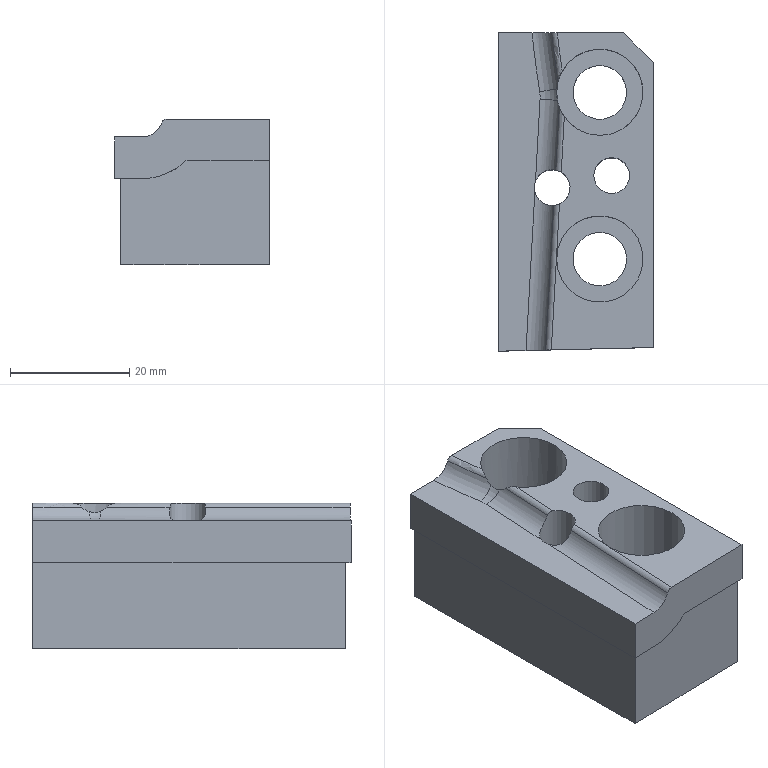Part | NX | features solid 2 | 1 solid | 27 faces | box 26 x 53.487 x 24.5 mm | volume 23516 mm3 | plane 12 | cylinder 10 | torus 3 | spline 2 | commonest cylinder face diameters 2 x2 6.001 x2 7 x2 9 x2 14.5 x2
STEP:
#1=CARTESIAN_POINT('',(636.878,-88.728,-8.5));
#2=VERTEX_POINT('',#1);
#3=CARTESIAN_POINT('',(636.878,-88.728,-23.));
#4=VERTEX_POINT('',#3);
#5=CARTESIAN_POINT('',(636.878,-88.728,-58.5));
#6=DIRECTION('',(0.,0.,1.));
#7=VECTOR('',#6,1000.);
#8=LINE('',#5,#7);
#9=EDGE_CURVE('',#2,#4,#8,.F.);
#10=ORIENTED_EDGE('',*,*,#9,.F.);
#11=CARTESIAN_POINT('',(636.878,-36.265,-8.5));
#12=VERTEX_POINT('',#11);
#13=CARTESIAN_POINT('',(636.878,-73.265,-8.5));
#14=DIRECTION('',(0.,-1.,0.));
#15=VECTOR('',#14,1000.);
#16=LINE('',#13,#15);
#17=EDGE_CURVE('',#12,#2,#16,.T.);
#18=ORIENTED_EDGE('',*,*,#17,.F.);
#19=CARTESIAN_POINT('',(636.878,-36.265,-23.));
#20=VERTEX_POINT('',#19);
#21=CARTESIAN_POINT('',(636.878,-36.265,-5.));
#22=DIRECTION('',(0.,0.,1.));
#23=VECTOR('',#22,1000.);
#24=LINE('',#21,#23);
#25=EDGE_CURVE('',#20,#12,#24,.T.);
#26=ORIENTED_EDGE('',*,*,#25,.F.);
#27=CARTESIAN_POINT('',(636.878,-73.265,-23.));
#28=DIRECTION('',(0.,1.,0.));
#29=VECTOR('',#28,1000.);
#30=LINE('',#27,#29);
#31=EDGE_CURVE('',#20,#4,#30,.F.);
#32=ORIENTED_EDGE('',*,*,#31,.T.);
#33=EDGE_LOOP('',(#10,#18,#26,#32));
#34=FACE_BOUND('',#33,.T.);
#35=CARTESIAN_POINT('',(636.878,-73.265,-5.));
#36=DIRECTION('',(1.,0.,0.));
#37=DIRECTION('',(0.,0.,-1.));
#38=AXIS2_PLACEMENT_3D('',#35,#36,#37);
#39=PLANE('',#38);
#40=ADVANCED_FACE('',(#34),#39,.F.);
#41=CARTESIAN_POINT('',(635.878,-89.752,-8.5));
#42=VERTEX_POINT('',#41);
#43=CARTESIAN_POINT('',(635.878,-89.752,-1.5));
#44=VERTEX_POINT('',#43);
#45=CARTESIAN_POINT('',(635.878,-89.752,22.));
#46=DIRECTION('',(0.,0.,1.));
#47=VECTOR('',#46,1000.);
#48=LINE('',#45,#47);
#49=EDGE_CURVE('',#42,#44,#48,.T.);
#50=ORIENTED_EDGE('',*,*,#49,.F.);
#51=CARTESIAN_POINT('',(661.878,-89.14,-5.5));
#52=VERTEX_POINT('',#51);
#53=CARTESIAN_POINT('',(635.878,-89.752,-8.5));
#54=CARTESIAN_POINT('',(636.986,-89.726,-8.499));
#55=CARTESIAN_POINT('',(639.207,-89.674,-8.501));
#56=CARTESIAN_POINT('',(641.968,-89.609,-8.497));
#57=CARTESIAN_POINT('',(643.879,-89.564,-7.982));
#58=CARTESIAN_POINT('',(644.896,-89.54,-7.513));
#59=CARTESIAN_POINT('',(645.651,-89.522,-7.153));
#60=CARTESIAN_POINT('',(646.405,-89.504,-6.758));
#61=CARTESIAN_POINT('',(647.005,-89.49,-6.173));
#62=CARTESIAN_POINT('',(647.588,-89.476,-5.535));
#63=CARTESIAN_POINT('',(648.442,-89.456,-5.389));
#64=CARTESIAN_POINT('',(649.272,-89.437,-5.531));
#65=CARTESIAN_POINT('',(650.112,-89.417,-5.53));
#66=CARTESIAN_POINT('',(650.952,-89.397,-5.477));
#67=CARTESIAN_POINT('',(652.073,-89.371,-5.506));
#68=CARTESIAN_POINT('',(653.473,-89.338,-5.497));
#69=CARTESIAN_POINT('',(655.715,-89.285,-5.503));
#70=CARTESIAN_POINT('',(658.516,-89.219,-5.499));
#71=CARTESIAN_POINT('',(660.757,-89.166,-5.5));
#72=CARTESIAN_POINT('',(661.878,-89.14,-5.5));
#73=B_SPLINE_CURVE_WITH_KNOTS('',3,(#53,#54,#55,#56,#57,#58,#59,#60,#61,#62,#63,#64,#65,#66,#67,#68,#69,#70,#71,#72),.UNSPECIFIED.,.F.,.F.,(4,1,1,1,1,1,1,1,1,1,1,1,1,1,1,1,1,4),(0.,0.003327,0.006654,0.008317,0.009149,0.009981,0.01081,0.01164,0.01248,0.01331,0.01414,0.01497,0.0158,0.01663,0.0183,0.01996,0.02329,0.02662),.UNSPECIFIED.);
#74=EDGE_CURVE('',#42,#52,#73,.T.);
#75=ORIENTED_EDGE('',*,*,#74,.T.);
#76=CARTESIAN_POINT('',(661.878,-89.14,1.5));
#77=VERTEX_POINT('',#76);
#78=CARTESIAN_POINT('',(661.878,-89.14,-9.));
#79=DIRECTION('',(0.,0.,-1.));
#80=VECTOR('',#79,1000.);
#81=LINE('',#78,#80);
#82=EDGE_CURVE('',#77,#52,#81,.T.);
#83=ORIENTED_EDGE('',*,*,#82,.F.);
#84=CARTESIAN_POINT('',(644.733,-89.543,1.5));
#85=VERTEX_POINT('',#84);
#86=CARTESIAN_POINT('',(315.699,-97.286,1.5));
#87=DIRECTION('',(0.9997,0.02352,0.));
#88=VECTOR('',#87,1000.);
#89=LINE('',#86,#88);
#90=EDGE_CURVE('',#85,#77,#89,.T.);
#91=ORIENTED_EDGE('',*,*,#90,.F.);
#92=CARTESIAN_POINT('',(643.788,-89.566,0.8333));
#93=VERTEX_POINT('',#92);
#94=CARTESIAN_POINT('',(644.733,-89.543,0.5));
#95=DIRECTION('',(0.02352,-0.9997,0.));
#96=DIRECTION('',(0.9997,0.02352,0.));
#97=AXIS2_PLACEMENT_3D('',#94,#95,#96);
#98=ELLIPSE('',#97,1.003,1.);
#99=EDGE_CURVE('',#93,#85,#98,.F.);
#100=ORIENTED_EDGE('',*,*,#99,.F.);
#101=CARTESIAN_POINT('',(640.478,-89.644,-1.5));
#102=VERTEX_POINT('',#101);
#103=CARTESIAN_POINT('',(640.478,-89.644,2.));
#104=DIRECTION('',(0.02352,-0.9997,0.));
#105=DIRECTION('',(0.9997,0.02352,0.));
#106=AXIS2_PLACEMENT_3D('',#103,#104,#105);
#107=ELLIPSE('',#106,3.511,3.5);
#108=EDGE_CURVE('',#93,#102,#107,.F.);
#109=ORIENTED_EDGE('',*,*,#108,.T.);
#110=CARTESIAN_POINT('',(315.699,-97.286,-1.5));
#111=DIRECTION('',(0.9997,0.02352,0.));
#112=VECTOR('',#111,1000.);
#113=LINE('',#110,#112);
#114=EDGE_CURVE('',#44,#102,#113,.T.);
#115=ORIENTED_EDGE('',*,*,#114,.F.);
#116=EDGE_LOOP('',(#50,#75,#83,#91,#100,#109,#115));
#117=FACE_BOUND('',#116,.T.);
#118=CARTESIAN_POINT('',(688.013,-88.525,22.));
#119=DIRECTION('',(0.02352,-0.9997,0.));
#120=DIRECTION('',(0.9997,0.02352,0.));
#121=AXIS2_PLACEMENT_3D('',#118,#119,#120);
#122=PLANE('',#121);
#123=ADVANCED_FACE('',(#117),#122,.T.);
#124=CARTESIAN_POINT('',(641.877,-62.265,-23.));
#125=VERTEX_POINT('',#124);
#126=CARTESIAN_POINT('',(644.878,-62.265,-23.));
#127=DIRECTION('',(0.,0.,-1.));
#128=DIRECTION('',(-1.,0.,0.));
#129=AXIS2_PLACEMENT_3D('',#126,#127,#128);
#130=CIRCLE('',#129,3.001);
#131=EDGE_CURVE('',#125,#125,#130,.T.);
#132=ORIENTED_EDGE('',*,*,#131,.F.);
#133=EDGE_LOOP('',(#132));
#134=FACE_BOUND('',#133,.T.);
#135=CARTESIAN_POINT('',(651.877,-60.265,-23.));
#136=VERTEX_POINT('',#135);
#137=CARTESIAN_POINT('',(654.878,-60.265,-23.));
#138=DIRECTION('',(0.,0.,-1.));
#139=DIRECTION('',(-1.,0.,0.));
#140=AXIS2_PLACEMENT_3D('',#137,#138,#139);
#141=CIRCLE('',#140,3.001);
#142=EDGE_CURVE('',#136,#136,#141,.T.);
#143=ORIENTED_EDGE('',*,*,#142,.F.);
#144=EDGE_LOOP('',(#143));
#145=FACE_BOUND('',#144,.T.);
#146=CARTESIAN_POINT('',(648.378,-46.265,-23.));
#147=VERTEX_POINT('',#146);
#148=CARTESIAN_POINT('',(652.878,-46.265,-23.));
#149=DIRECTION('',(0.,0.,-1.));
#150=DIRECTION('',(-1.,0.,0.));
#151=AXIS2_PLACEMENT_3D('',#148,#149,#150);
#152=CIRCLE('',#151,4.5);
#153=EDGE_CURVE('',#147,#147,#152,.F.);
#154=ORIENTED_EDGE('',*,*,#153,.T.);
#155=EDGE_LOOP('',(#154));
#156=FACE_BOUND('',#155,.T.);
#157=CARTESIAN_POINT('',(648.378,-74.265,-23.));
#158=VERTEX_POINT('',#157);
#159=CARTESIAN_POINT('',(652.878,-74.265,-23.));
#160=DIRECTION('',(0.,0.,-1.));
#161=DIRECTION('',(-1.,0.,0.));
#162=AXIS2_PLACEMENT_3D('',#159,#160,#161);
#163=CIRCLE('',#162,4.5);
#164=EDGE_CURVE('',#158,#158,#163,.F.);
#165=ORIENTED_EDGE('',*,*,#164,.T.);
#166=EDGE_LOOP('',(#165));
#167=FACE_BOUND('',#166,.T.);
#168=CARTESIAN_POINT('',(661.878,-88.14,-23.));
#169=VERTEX_POINT('',#168);
#170=CARTESIAN_POINT('',(636.878,-88.728,-23.));
#171=CARTESIAN_POINT('',(645.211,-88.532,-23.));
#172=CARTESIAN_POINT('',(653.544,-88.336,-23.));
#173=CARTESIAN_POINT('',(661.878,-88.14,-23.));
#174=B_SPLINE_CURVE_WITH_KNOTS('',3,(#170,#171,#172,#173),.UNSPECIFIED.,.F.,.F.,(4,4),(0.,0.02501),.UNSPECIFIED.);
#175=EDGE_CURVE('',#4,#169,#174,.T.);
#176=ORIENTED_EDGE('',*,*,#175,.F.);
#177=ORIENTED_EDGE('',*,*,#31,.F.);
#178=CARTESIAN_POINT('',(656.878,-36.265,-23.));
#179=VERTEX_POINT('',#178);
#180=CARTESIAN_POINT('',(658.878,-36.265,-23.));
#181=DIRECTION('',(1.,0.,0.));
#182=VECTOR('',#181,1000.);
#183=LINE('',#180,#182);
#184=EDGE_CURVE('',#179,#20,#183,.F.);
#185=ORIENTED_EDGE('',*,*,#184,.F.);
#186=CARTESIAN_POINT('',(661.878,-41.265,-23.));
#187=VERTEX_POINT('',#186);
#188=CARTESIAN_POINT('',(661.878,-41.265,-23.));
#189=DIRECTION('',(-0.7071,0.7071,0.));
#190=VECTOR('',#189,1000.);
#191=LINE('',#188,#190);
#192=EDGE_CURVE('',#179,#187,#191,.F.);
#193=ORIENTED_EDGE('',*,*,#192,.T.);
#194=CARTESIAN_POINT('',(661.878,-62.738,-23.));
#195=DIRECTION('',(0.,1.,0.));
#196=VECTOR('',#195,1000.);
#197=LINE('',#194,#196);
#198=EDGE_CURVE('',#187,#169,#197,.F.);
#199=ORIENTED_EDGE('',*,*,#198,.T.);
#200=EDGE_LOOP('',(#176,#177,#185,#193,#199));
#201=FACE_BOUND('',#200,.T.);
#202=CARTESIAN_POINT('',(699.237,0.,-23.));
#203=DIRECTION('',(0.,0.,-1.));
#204=DIRECTION('',(-1.,0.,0.));
#205=AXIS2_PLACEMENT_3D('',#202,#203,#204);
#206=PLANE('',#205);
#207=ADVANCED_FACE('',(#134,#145,#156,#167,#201),#206,.T.);
#208=CARTESIAN_POINT('',(635.878,-88.752,-8.5));
#209=VERTEX_POINT('',#208);
#210=CARTESIAN_POINT('',(635.878,-88.752,-8.5));
#211=CARTESIAN_POINT('',(636.211,-88.744,-8.5));
#212=CARTESIAN_POINT('',(636.544,-88.736,-8.5));
#213=CARTESIAN_POINT('',(636.878,-88.728,-8.5));
#214=B_SPLINE_CURVE_WITH_KNOTS('',3,(#210,#211,#212,#213),.UNSPECIFIED.,.F.,.F.,(4,4),(0.,1.),.UNSPECIFIED.);
#215=EDGE_CURVE('',#209,#2,#214,.T.);
#216=ORIENTED_EDGE('',*,*,#215,.F.);
#217=CARTESIAN_POINT('',(635.878,-36.265,-8.5));
#218=VERTEX_POINT('',#217);
#219=CARTESIAN_POINT('',(635.878,-73.265,-8.5));
#220=DIRECTION('',(0.,-1.,0.));
#221=VECTOR('',#220,1000.);
#222=LINE('',#219,#221);
#223=EDGE_CURVE('',#209,#218,#222,.F.);
#224=ORIENTED_EDGE('',*,*,#223,.T.);
#225=CARTESIAN_POINT('',(658.878,-36.265,-8.5));
#226=DIRECTION('',(-1.,0.,0.));
#227=VECTOR('',#226,1000.);
#228=LINE('',#225,#227);
#229=EDGE_CURVE('',#12,#218,#228,.T.);
#230=ORIENTED_EDGE('',*,*,#229,.F.);
#231=ORIENTED_EDGE('',*,*,#17,.T.);
#232=EDGE_LOOP('',(#216,#224,#230,#231));
#233=FACE_BOUND('',#232,.T.);
#234=CARTESIAN_POINT('',(639.36,-63.009,-8.5));
#235=DIRECTION('',(0.,0.,1.));
#236=DIRECTION('',(1.,0.,0.));
#237=AXIS2_PLACEMENT_3D('',#234,#235,#236);
#238=PLANE('',#237);
#239=ADVANCED_FACE('',(#233),#238,.F.);
#240=CARTESIAN_POINT('',(635.878,-89.751,-8.5));
#241=DIRECTION('',(0.,1.,0.00001958));
#242=VECTOR('',#241,1000.);
#243=LINE('',#240,#242);
#244=EDGE_CURVE('',#42,#209,#243,.T.);
#245=ORIENTED_EDGE('',*,*,#244,.F.);
#246=ORIENTED_EDGE('',*,*,#49,.T.);
#247=CARTESIAN_POINT('',(635.878,-36.265,-1.5));
#248=VERTEX_POINT('',#247);
#249=CARTESIAN_POINT('',(635.878,343.366,-1.5));
#250=DIRECTION('',(0.,1.,0.));
#251=VECTOR('',#250,1000.);
#252=LINE('',#249,#251);
#253=EDGE_CURVE('',#44,#248,#252,.T.);
#254=ORIENTED_EDGE('',*,*,#253,.T.);
#255=CARTESIAN_POINT('',(635.878,-36.265,-5.));
#256=DIRECTION('',(0.,0.,1.));
#257=VECTOR('',#256,1000.);
#258=LINE('',#255,#257);
#259=EDGE_CURVE('',#218,#248,#258,.T.);
#260=ORIENTED_EDGE('',*,*,#259,.F.);
#261=ORIENTED_EDGE('',*,*,#223,.F.);
#262=EDGE_LOOP('',(#245,#246,#254,#260,#261));
#263=FACE_BOUND('',#262,.T.);
#264=CARTESIAN_POINT('',(635.878,-73.265,-5.));
#265=DIRECTION('',(1.,0.,0.));
#266=DIRECTION('',(0.,0.,-1.));
#267=AXIS2_PLACEMENT_3D('',#264,#265,#266);
#268=PLANE('',#267);
#269=ADVANCED_FACE('',(#263),#268,.F.);
#270=CARTESIAN_POINT('',(661.878,-88.14,-5.5));
#271=VERTEX_POINT('',#270);
#272=CARTESIAN_POINT('',(661.878,-88.14,-55.5));
#273=DIRECTION('',(0.,0.,1.));
#274=VECTOR('',#273,1000.);
#275=LINE('',#272,#274);
#276=EDGE_CURVE('',#169,#271,#275,.T.);
#277=ORIENTED_EDGE('',*,*,#276,.F.);
#278=ORIENTED_EDGE('',*,*,#198,.F.);
#279=CARTESIAN_POINT('',(661.878,-41.265,1.5));
#280=VERTEX_POINT('',#279);
#281=CARTESIAN_POINT('',(661.878,-41.265,1.51));
#282=DIRECTION('',(0.,0.,1.));
#283=VECTOR('',#282,1000.);
#284=LINE('',#281,#283);
#285=EDGE_CURVE('',#187,#280,#284,.T.);
#286=ORIENTED_EDGE('',*,*,#285,.T.);
#287=CARTESIAN_POINT('',(661.878,343.366,1.5));
#288=DIRECTION('',(0.,1.,0.));
#289=VECTOR('',#288,1000.);
#290=LINE('',#287,#289);
#291=EDGE_CURVE('',#77,#280,#290,.T.);
#292=ORIENTED_EDGE('',*,*,#291,.F.);
#293=ORIENTED_EDGE('',*,*,#82,.T.);
#294=CARTESIAN_POINT('',(661.878,-88.14,-5.5));
#295=CARTESIAN_POINT('',(661.878,-88.473,-5.5));
#296=CARTESIAN_POINT('',(661.878,-88.807,-5.5));
#297=CARTESIAN_POINT('',(661.878,-89.14,-5.5));
#298=B_SPLINE_CURVE_WITH_KNOTS('',3,(#294,#295,#296,#297),.UNSPECIFIED.,.F.,.F.,(4,4),(0.,0.001),.UNSPECIFIED.);
#299=EDGE_CURVE('',#271,#52,#298,.T.);
#300=ORIENTED_EDGE('',*,*,#299,.F.);
#301=EDGE_LOOP('',(#277,#278,#286,#292,#293,#300));
#302=FACE_BOUND('',#301,.T.);
#303=CARTESIAN_POINT('',(661.878,-62.738,-9.));
#304=DIRECTION('',(1.,0.,0.));
#305=DIRECTION('',(0.,0.,-1.));
#306=AXIS2_PLACEMENT_3D('',#303,#304,#305);
#307=PLANE('',#306);
#308=ADVANCED_FACE('',(#302),#307,.T.);
#309=ORIENTED_EDGE('',*,*,#25,.T.);
#310=ORIENTED_EDGE('',*,*,#229,.T.);
#311=ORIENTED_EDGE('',*,*,#259,.T.);
#312=CARTESIAN_POINT('',(641.479,-36.265,-1.5));
#313=VERTEX_POINT('',#312);
#314=CARTESIAN_POINT('',(305.33,-36.265,-1.5));
#315=DIRECTION('',(1.,0.,0.));
#316=VECTOR('',#315,1000.);
#317=LINE('',#314,#316);
#318=EDGE_CURVE('',#248,#313,#317,.T.);
#319=ORIENTED_EDGE('',*,*,#318,.T.);
#320=CARTESIAN_POINT('',(644.798,-36.265,0.8333));
#321=VERTEX_POINT('',#320);
#322=CARTESIAN_POINT('',(644.798,-36.265,0.8333));
#323=CARTESIAN_POINT('',(644.311,-36.265,-0.5365));
#324=CARTESIAN_POINT('',(642.932,-36.265,-1.5));
#325=CARTESIAN_POINT('',(641.479,-36.265,-1.5));
#326=B_SPLINE_CURVE_WITH_KNOTS('',3,(#322,#323,#324,#325),.UNSPECIFIED.,.F.,.F.,(4,4),(0.,0.0043),.UNSPECIFIED.);
#327=EDGE_CURVE('',#321,#313,#326,.T.);
#328=ORIENTED_EDGE('',*,*,#327,.F.);
#329=CARTESIAN_POINT('',(645.747,-36.265,1.5));
#330=VERTEX_POINT('',#329);
#331=CARTESIAN_POINT('',(644.798,-36.265,0.8333));
#332=CARTESIAN_POINT('',(644.938,-36.265,1.225));
#333=CARTESIAN_POINT('',(645.331,-36.265,1.5));
#334=CARTESIAN_POINT('',(645.747,-36.265,1.5));
#335=B_SPLINE_CURVE_WITH_KNOTS('',3,(#331,#332,#333,#334),.UNSPECIFIED.,.F.,.F.,(4,4),(0.,0.001229),.UNSPECIFIED.);
#336=EDGE_CURVE('',#321,#330,#335,.T.);
#337=ORIENTED_EDGE('',*,*,#336,.T.);
#338=CARTESIAN_POINT('',(656.878,-36.265,1.5));
#339=VERTEX_POINT('',#338);
#340=CARTESIAN_POINT('',(305.33,-36.265,1.5));
#341=DIRECTION('',(1.,0.,0.));
#342=VECTOR('',#341,1000.);
#343=LINE('',#340,#342);
#344=EDGE_CURVE('',#330,#339,#343,.T.);
#345=ORIENTED_EDGE('',*,*,#344,.T.);
#346=CARTESIAN_POINT('',(656.878,-36.265,-23.));
#347=DIRECTION('',(0.,0.,-1.));
#348=VECTOR('',#347,1000.);
#349=LINE('',#346,#348);
#350=EDGE_CURVE('',#339,#179,#349,.T.);
#351=ORIENTED_EDGE('',*,*,#350,.T.);
#352=ORIENTED_EDGE('',*,*,#184,.T.);
#353=EDGE_LOOP('',(#309,#310,#311,#319,#328,#337,#345,#351,#352));
#354=FACE_BOUND('',#353,.T.);
#355=CARTESIAN_POINT('',(658.878,-36.265,-5.));
#356=DIRECTION('',(0.,-1.,0.));
#357=DIRECTION('',(0.,0.,-1.));
#358=AXIS2_PLACEMENT_3D('',#355,#356,#357);
#359=PLANE('',#358);
#360=ADVANCED_FACE('',(#354),#359,.F.);
#361=ORIENTED_EDGE('',*,*,#350,.F.);
#362=CARTESIAN_POINT('',(291.288,329.324,1.5));
#363=DIRECTION('',(-0.7071,0.7071,0.));
#364=VECTOR('',#363,1000.);
#365=LINE('',#362,#364);
#366=EDGE_CURVE('',#280,#339,#365,.T.);
#367=ORIENTED_EDGE('',*,*,#366,.F.);
#368=ORIENTED_EDGE('',*,*,#285,.F.);
#369=ORIENTED_EDGE('',*,*,#192,.F.);
#370=EDGE_LOOP('',(#361,#367,#368,#369));
#371=FACE_BOUND('',#370,.T.);
#372=CARTESIAN_POINT('',(661.878,-41.265,-9.));
#373=DIRECTION('',(0.7071,0.7071,0.));
#374=DIRECTION('',(0.,0.,-1.));
#375=AXIS2_PLACEMENT_3D('',#372,#373,#374);
#376=PLANE('',#375);
#377=ADVANCED_FACE('',(#371),#376,.T.);
#378=CARTESIAN_POINT('',(645.628,-74.265,-13.));
#379=VERTEX_POINT('',#378);
#380=CARTESIAN_POINT('',(652.878,-74.265,-13.));
#381=DIRECTION('',(0.,0.,-1.));
#382=DIRECTION('',(-1.,0.,0.));
#383=AXIS2_PLACEMENT_3D('',#380,#381,#382);
#384=CIRCLE('',#383,7.25);
#385=EDGE_CURVE('',#379,#379,#384,.T.);
#386=ORIENTED_EDGE('',*,*,#385,.T.);
#387=EDGE_LOOP('',(#386));
#388=FACE_BOUND('',#387,.T.);
#389=CARTESIAN_POINT('',(660.128,-74.265,1.5));
#390=VERTEX_POINT('',#389);
#391=CARTESIAN_POINT('',(652.878,-74.265,1.5));
#392=DIRECTION('',(0.,0.,1.));
#393=DIRECTION('',(1.,0.,0.));
#394=AXIS2_PLACEMENT_3D('',#391,#392,#393);
#395=CIRCLE('',#394,7.25);
#396=EDGE_CURVE('',#390,#390,#395,.F.);
#397=ORIENTED_EDGE('',*,*,#396,.F.);
#398=EDGE_LOOP('',(#397));
#399=FACE_BOUND('',#398,.T.);
#400=CARTESIAN_POINT('',(652.878,-74.265,77.));
#401=DIRECTION('',(0.,0.,-1.));
#402=DIRECTION('',(-1.,0.,0.));
#403=AXIS2_PLACEMENT_3D('',#400,#401,#402);
#404=CYLINDRICAL_SURFACE('',#403,7.25);
#405=ADVANCED_FACE('',(#388,#399),#404,.F.);
#406=ORIENTED_EDGE('',*,*,#142,.T.);
#407=EDGE_LOOP('',(#406));
#408=FACE_BOUND('',#407,.T.);
#409=CARTESIAN_POINT('',(657.878,-60.265,1.5));
#410=VERTEX_POINT('',#409);
#411=CARTESIAN_POINT('',(654.878,-60.265,1.5));
#412=DIRECTION('',(0.,0.,1.));
#413=DIRECTION('',(1.,0.,0.));
#414=AXIS2_PLACEMENT_3D('',#411,#412,#413);
#415=CIRCLE('',#414,3.001);
#416=EDGE_CURVE('',#410,#410,#415,.F.);
#417=ORIENTED_EDGE('',*,*,#416,.F.);
#418=EDGE_LOOP('',(#417));
#419=FACE_BOUND('',#418,.T.);
#420=CARTESIAN_POINT('',(654.878,-60.265,-133.));
#421=DIRECTION('',(0.,0.,1.));
#422=DIRECTION('',(1.,0.,0.));
#423=AXIS2_PLACEMENT_3D('',#420,#421,#422);
#424=CYLINDRICAL_SURFACE('',#423,3.001);
#425=ADVANCED_FACE('',(#408,#419),#424,.F.);
#426=ORIENTED_EDGE('',*,*,#131,.T.);
#427=EDGE_LOOP('',(#426));
#428=FACE_BOUND('',#427,.T.);
#429=CARTESIAN_POINT('',(646.4,-59.679,1.5));
#430=VERTEX_POINT('',#429);
#431=CARTESIAN_POINT('',(646.103,-65.004,1.5));
#432=VERTEX_POINT('',#431);
#433=CARTESIAN_POINT('',(644.878,-62.265,1.5));
#434=DIRECTION('',(0.,0.,1.));
#435=DIRECTION('',(1.,0.,0.));
#436=AXIS2_PLACEMENT_3D('',#433,#434,#435);
#437=CIRCLE('',#436,3.001);
#438=EDGE_CURVE('',#430,#432,#437,.F.);
#439=ORIENTED_EDGE('',*,*,#438,.F.);
#440=CARTESIAN_POINT('',(645.475,-59.325,0.8333));
#441=VERTEX_POINT('',#440);
#442=CARTESIAN_POINT('',(645.475,-59.325,0.8333));
#443=CARTESIAN_POINT('',(645.617,-59.354,1.238));
#444=CARTESIAN_POINT('',(646.03,-59.462,1.5));
#445=CARTESIAN_POINT('',(646.4,-59.679,1.5));
#446=B_SPLINE_CURVE_WITH_KNOTS('',3,(#442,#443,#444,#445),.UNSPECIFIED.,.F.,.F.,(4,4),(0.,0.001272),.UNSPECIFIED.);
#447=EDGE_CURVE('',#441,#430,#446,.T.);
#448=ORIENTED_EDGE('',*,*,#447,.F.);
#449=CARTESIAN_POINT('',(642.064,-61.222,-1.5));
#450=VERTEX_POINT('',#449);
#451=CARTESIAN_POINT('',(645.475,-59.325,0.8333));
#452=CARTESIAN_POINT('',(645.185,-59.266,0.004989));
#453=CARTESIAN_POINT('',(643.863,-59.084,-1.42));
#454=CARTESIAN_POINT('',(642.371,-60.395,-1.5));
#455=CARTESIAN_POINT('',(642.064,-61.222,-1.5));
#456=B_SPLINE_CURVE_WITH_KNOTS('',3,(#451,#452,#453,#454,#455),.UNSPECIFIED.,.F.,.F.,(4,1,4),(0.,0.002605,0.005209),.UNSPECIFIED.);
#457=EDGE_CURVE('',#441,#450,#456,.T.);
#458=ORIENTED_EDGE('',*,*,#457,.T.);
#459=CARTESIAN_POINT('',(641.966,-62.989,-1.5));
#460=VERTEX_POINT('',#459);
#461=CARTESIAN_POINT('',(644.878,-62.265,-1.5));
#462=DIRECTION('',(0.,0.,1.));
#463=DIRECTION('',(1.,0.,0.));
#464=AXIS2_PLACEMENT_3D('',#461,#462,#463);
#465=CIRCLE('',#464,3.001);
#466=EDGE_CURVE('',#460,#450,#465,.F.);
#467=ORIENTED_EDGE('',*,*,#466,.F.);
#468=CARTESIAN_POINT('',(645.144,-65.254,0.8333));
#469=VERTEX_POINT('',#468);
#470=CARTESIAN_POINT('',(641.966,-62.989,-1.5));
#471=CARTESIAN_POINT('',(642.178,-63.843,-1.5));
#472=CARTESIAN_POINT('',(643.499,-65.306,-1.43));
#473=CARTESIAN_POINT('',(644.85,-65.28,0.004986));
#474=CARTESIAN_POINT('',(645.144,-65.254,0.8333));
#475=B_SPLINE_CURVE_WITH_KNOTS('',3,(#470,#471,#472,#473,#474),.UNSPECIFIED.,.F.,.F.,(4,1,4),(0.,0.002605,0.005211),.UNSPECIFIED.);
#476=EDGE_CURVE('',#460,#469,#475,.T.);
#477=ORIENTED_EDGE('',*,*,#476,.T.);
#478=CARTESIAN_POINT('',(646.103,-65.004,1.5));
#479=CARTESIAN_POINT('',(645.711,-65.18,1.5));
#480=CARTESIAN_POINT('',(645.289,-65.241,1.238));
#481=CARTESIAN_POINT('',(645.144,-65.254,0.8333));
#482=B_SPLINE_CURVE_WITH_KNOTS('',3,(#478,#479,#480,#481),.UNSPECIFIED.,.F.,.F.,(4,4),(0.,0.001272),.UNSPECIFIED.);
#483=EDGE_CURVE('',#432,#469,#482,.T.);
#484=ORIENTED_EDGE('',*,*,#483,.F.);
#485=EDGE_LOOP('',(#439,#448,#458,#467,#477,#484));
#486=FACE_BOUND('',#485,.T.);
#487=CARTESIAN_POINT('',(644.878,-62.265,-133.));
#488=DIRECTION('',(0.,0.,1.));
#489=DIRECTION('',(1.,0.,0.));
#490=AXIS2_PLACEMENT_3D('',#487,#488,#489);
#491=CYLINDRICAL_SURFACE('',#490,3.001);
#492=ADVANCED_FACE('',(#428,#486),#491,.F.);
#493=CARTESIAN_POINT('',(645.628,-46.265,-13.));
#494=VERTEX_POINT('',#493);
#495=CARTESIAN_POINT('',(652.878,-46.265,-13.));
#496=DIRECTION('',(0.,0.,-1.));
#497=DIRECTION('',(-1.,0.,0.));
#498=AXIS2_PLACEMENT_3D('',#495,#496,#497);
#499=CIRCLE('',#498,7.25);
#500=EDGE_CURVE('',#494,#494,#499,.T.);
#501=ORIENTED_EDGE('',*,*,#500,.T.);
#502=EDGE_LOOP('',(#501));
#503=FACE_BOUND('',#502,.T.);
#504=CARTESIAN_POINT('',(645.855,-44.464,0.8333));
#505=VERTEX_POINT('',#504);
#506=CARTESIAN_POINT('',(645.649,-45.708,0.05746));
#507=VERTEX_POINT('',#506);
#508=CARTESIAN_POINT('',(645.855,-44.464,0.8333));
#509=CARTESIAN_POINT('',(645.77,-44.794,0.4606));
#510=CARTESIAN_POINT('',(645.686,-45.234,0.2191));
#511=CARTESIAN_POINT('',(645.649,-45.708,0.05746));
#512=B_SPLINE_CURVE_WITH_KNOTS('',3,(#508,#509,#510,#511),.UNSPECIFIED.,.F.,.F.,(4,4),(0.,0.001485),.UNSPECIFIED.);
#513=EDGE_CURVE('',#505,#507,#512,.T.);
#514=ORIENTED_EDGE('',*,*,#513,.T.);
#515=CARTESIAN_POINT('',(645.753,-47.606,0.07633));
#516=VERTEX_POINT('',#515);
#517=CARTESIAN_POINT('',(645.649,-45.708,0.05746));
#518=CARTESIAN_POINT('',(645.602,-46.325,-0.1527));
#519=CARTESIAN_POINT('',(645.639,-47.003,-0.147));
#520=CARTESIAN_POINT('',(645.753,-47.606,0.07633));
#521=B_SPLINE_CURVE_WITH_KNOTS('',3,(#517,#518,#519,#520),.UNSPECIFIED.,.F.,.F.,(4,4),(0.,0.001931),.UNSPECIFIED.);
#522=EDGE_CURVE('',#507,#516,#521,.T.);
#523=ORIENTED_EDGE('',*,*,#522,.T.);
#524=CARTESIAN_POINT('',(646.066,-48.747,0.8333));
#525=VERTEX_POINT('',#524);
#526=CARTESIAN_POINT('',(645.753,-47.606,0.07633));
#527=CARTESIAN_POINT('',(645.835,-48.045,0.2389));
#528=CARTESIAN_POINT('',(645.957,-48.447,0.4784));
#529=CARTESIAN_POINT('',(646.066,-48.747,0.8333));
#530=B_SPLINE_CURVE_WITH_KNOTS('',3,(#526,#527,#528,#529),.UNSPECIFIED.,.F.,.F.,(4,4),(0.,0.001411),.UNSPECIFIED.);
#531=EDGE_CURVE('',#516,#525,#530,.T.);
#532=ORIENTED_EDGE('',*,*,#531,.T.);
#533=CARTESIAN_POINT('',(646.918,-50.394,1.5));
#534=VERTEX_POINT('',#533);
#535=CARTESIAN_POINT('',(646.918,-50.394,1.5));
#536=CARTESIAN_POINT('',(646.725,-50.115,1.5));
#537=CARTESIAN_POINT('',(646.388,-49.549,1.372));
#538=CARTESIAN_POINT('',(646.144,-48.961,1.088));
#539=CARTESIAN_POINT('',(646.066,-48.747,0.8333));
#540=B_SPLINE_CURVE_WITH_KNOTS('',3,(#535,#536,#537,#538,#539),.UNSPECIFIED.,.F.,.F.,(4,1,4),(0.,0.001004,0.002008),.UNSPECIFIED.);
#541=EDGE_CURVE('',#534,#525,#540,.T.);
#542=ORIENTED_EDGE('',*,*,#541,.F.);
#543=CARTESIAN_POINT('',(646.556,-42.716,1.5));
#544=VERTEX_POINT('',#543);
#545=CARTESIAN_POINT('',(652.878,-46.265,1.5));
#546=DIRECTION('',(0.,0.,1.));
#547=DIRECTION('',(1.,0.,0.));
#548=AXIS2_PLACEMENT_3D('',#545,#546,#547);
#549=CIRCLE('',#548,7.25);
#550=EDGE_CURVE('',#544,#534,#549,.F.);
#551=ORIENTED_EDGE('',*,*,#550,.F.);
#552=CARTESIAN_POINT('',(645.855,-44.464,0.8333));
#553=CARTESIAN_POINT('',(645.913,-44.237,1.09));
#554=CARTESIAN_POINT('',(646.101,-43.623,1.37));
#555=CARTESIAN_POINT('',(646.388,-43.015,1.5));
#556=CARTESIAN_POINT('',(646.556,-42.716,1.5));
#557=B_SPLINE_CURVE_WITH_KNOTS('',3,(#552,#553,#554,#555,#556),.UNSPECIFIED.,.F.,.F.,(4,1,4),(0.,0.001021,0.002043),.UNSPECIFIED.);
#558=EDGE_CURVE('',#505,#544,#557,.T.);
#559=ORIENTED_EDGE('',*,*,#558,.F.);
#560=EDGE_LOOP('',(#514,#523,#532,#542,#551,#559));
#561=FACE_BOUND('',#560,.T.);
#562=CARTESIAN_POINT('',(652.878,-46.265,77.));
#563=DIRECTION('',(0.,0.,-1.));
#564=DIRECTION('',(-1.,0.,0.));
#565=AXIS2_PLACEMENT_3D('',#562,#563,#564);
#566=CYLINDRICAL_SURFACE('',#565,7.25);
#567=ADVANCED_FACE('',(#503,#561),#566,.F.);
#568=CARTESIAN_POINT('',(648.378,-74.265,-13.));
#569=VERTEX_POINT('',#568);
#570=CARTESIAN_POINT('',(652.878,-74.265,-13.));
#571=DIRECTION('',(0.,0.,-1.));
#572=DIRECTION('',(-1.,0.,0.));
#573=AXIS2_PLACEMENT_3D('',#570,#571,#572);
#574=CIRCLE('',#573,4.5);
#575=EDGE_CURVE('',#569,#569,#574,.T.);
#576=ORIENTED_EDGE('',*,*,#575,.T.);
#577=EDGE_LOOP('',(#576));
#578=FACE_BOUND('',#577,.T.);
#579=ORIENTED_EDGE('',*,*,#385,.F.);
#580=EDGE_LOOP('',(#579));
#581=FACE_BOUND('',#580,.T.);
#582=CARTESIAN_POINT('',(648.475,67.468,-13.));
#583=DIRECTION('',(0.,0.,-1.));
#584=DIRECTION('',(-1.,0.,0.));
#585=AXIS2_PLACEMENT_3D('',#582,#583,#584);
#586=PLANE('',#585);
#587=ADVANCED_FACE('',(#578,#581),#586,.F.);
#588=CARTESIAN_POINT('',(648.378,-46.265,-13.));
#589=VERTEX_POINT('',#588);
#590=CARTESIAN_POINT('',(652.878,-46.265,-13.));
#591=DIRECTION('',(0.,0.,-1.));
#592=DIRECTION('',(-1.,0.,0.));
#593=AXIS2_PLACEMENT_3D('',#590,#591,#592);
#594=CIRCLE('',#593,4.5);
#595=EDGE_CURVE('',#589,#589,#594,.T.);
#596=ORIENTED_EDGE('',*,*,#595,.T.);
#597=EDGE_LOOP('',(#596));
#598=FACE_BOUND('',#597,.T.);
#599=ORIENTED_EDGE('',*,*,#500,.F.);
#600=EDGE_LOOP('',(#599));
#601=FACE_BOUND('',#600,.T.);
#602=CARTESIAN_POINT('',(648.475,95.468,-13.));
#603=DIRECTION('',(0.,0.,-1.));
#604=DIRECTION('',(-1.,0.,0.));
#605=AXIS2_PLACEMENT_3D('',#602,#603,#604);
#606=PLANE('',#605);
#607=ADVANCED_FACE('',(#598,#601),#606,.F.);
#608=ORIENTED_EDGE('',*,*,#595,.F.);
#609=EDGE_LOOP('',(#608));
#610=FACE_BOUND('',#609,.T.);
#611=ORIENTED_EDGE('',*,*,#153,.F.);
#612=EDGE_LOOP('',(#611));
#613=FACE_BOUND('',#612,.T.);
#614=CARTESIAN_POINT('',(652.878,-46.265,-42.298));
#615=DIRECTION('',(0.,0.,1.));
#616=DIRECTION('',(1.,0.,0.));
#617=AXIS2_PLACEMENT_3D('',#614,#615,#616);
#618=CYLINDRICAL_SURFACE('',#617,4.5);
#619=ADVANCED_FACE('',(#610,#613),#618,.F.);
#620=ORIENTED_EDGE('',*,*,#575,.F.);
#621=EDGE_LOOP('',(#620));
#622=FACE_BOUND('',#621,.T.);
#623=ORIENTED_EDGE('',*,*,#164,.F.);
#624=EDGE_LOOP('',(#623));
#625=FACE_BOUND('',#624,.T.);
#626=CARTESIAN_POINT('',(652.878,-74.265,-42.298));
#627=DIRECTION('',(0.,0.,1.));
#628=DIRECTION('',(1.,0.,0.));
#629=AXIS2_PLACEMENT_3D('',#626,#627,#628);
#630=CYLINDRICAL_SURFACE('',#629,4.5);
#631=ADVANCED_FACE('',(#622,#625),#630,.F.);
#632=CARTESIAN_POINT('',(645.555,-74.81,1.5));
#633=DIRECTION('',(0.05572,0.9984,0.));
#634=VECTOR('',#633,1000.);
#635=LINE('',#632,#634);
#636=EDGE_CURVE('',#432,#85,#635,.F.);
#637=ORIENTED_EDGE('',*,*,#636,.F.);
#638=ORIENTED_EDGE('',*,*,#483,.T.);
#639=CARTESIAN_POINT('',(643.775,-89.8,0.8333));
#640=DIRECTION('',(0.05572,0.9984,0.));
#641=VECTOR('',#640,1000.);
#642=LINE('',#639,#641);
#643=EDGE_CURVE('',#469,#93,#642,.F.);
#644=ORIENTED_EDGE('',*,*,#643,.T.);
#645=ORIENTED_EDGE('',*,*,#99,.T.);
#646=EDGE_LOOP('',(#637,#638,#644,#645));
#647=FACE_BOUND('',#646,.T.);
#648=CARTESIAN_POINT('',(644.716,-89.852,0.5));
#649=DIRECTION('',(0.05572,0.9984,0.));
#650=DIRECTION('',(0.9413,-0.05253,-0.3333));
#651=AXIS2_PLACEMENT_3D('',#648,#649,#650);
#652=CYLINDRICAL_SURFACE('',#651,1.);
#653=ADVANCED_FACE('',(#647),#652,.T.);
#654=ORIENTED_EDGE('',*,*,#476,.F.);
#655=CARTESIAN_POINT('',(640.256,-93.637,-1.5));
#656=DIRECTION('',(0.05572,0.9984,0.));
#657=VECTOR('',#656,1000.);
#658=LINE('',#655,#657);
#659=EDGE_CURVE('',#102,#460,#658,.T.);
#660=ORIENTED_EDGE('',*,*,#659,.F.);
#661=ORIENTED_EDGE('',*,*,#108,.F.);
#662=ORIENTED_EDGE('',*,*,#643,.F.);
#663=EDGE_LOOP('',(#654,#660,#661,#662));
#664=FACE_BOUND('',#663,.T.);
#665=CARTESIAN_POINT('',(640.256,-93.637,2.));
#666=DIRECTION('',(0.05572,0.9984,0.));
#667=DIRECTION('',(-0.9413,0.05253,0.3333));
#668=AXIS2_PLACEMENT_3D('',#665,#666,#667);
#669=CYLINDRICAL_SURFACE('',#668,3.5);
#670=ADVANCED_FACE('',(#664),#669,.F.);
#671=ORIENTED_EDGE('',*,*,#659,.T.);
#672=ORIENTED_EDGE('',*,*,#466,.T.);
#673=CARTESIAN_POINT('',(642.833,-47.443,-1.5));
#674=VERTEX_POINT('',#673);
#675=CARTESIAN_POINT('',(640.256,-93.637,-1.5));
#676=DIRECTION('',(0.05572,0.9984,0.));
#677=VECTOR('',#676,1000.);
#678=LINE('',#675,#677);
#679=EDGE_CURVE('',#450,#674,#678,.T.);
#680=ORIENTED_EDGE('',*,*,#679,.T.);
#681=CARTESIAN_POINT('',(642.771,-46.148,-1.5));
#682=VERTEX_POINT('',#681);
#683=CARTESIAN_POINT('',(636.586,-47.094,-1.5));
#684=DIRECTION('',(0.,0.,1.));
#685=DIRECTION('',(0.,-1.,0.));
#686=AXIS2_PLACEMENT_3D('',#683,#684,#685);
#687=CIRCLE('',#686,6.257);
#688=EDGE_CURVE('',#674,#682,#687,.T.);
#689=ORIENTED_EDGE('',*,*,#688,.T.);
#690=CARTESIAN_POINT('',(869.499,-11.474,-1.5));
#691=DIRECTION('',(0.,0.,1.));
#692=DIRECTION('',(0.,-1.,0.));
#693=AXIS2_PLACEMENT_3D('',#690,#691,#692);
#694=CIRCLE('',#693,229.364);
#695=EDGE_CURVE('',#682,#313,#694,.F.);
#696=ORIENTED_EDGE('',*,*,#695,.T.);
#697=ORIENTED_EDGE('',*,*,#318,.F.);
#698=ORIENTED_EDGE('',*,*,#253,.F.);
#699=ORIENTED_EDGE('',*,*,#114,.T.);
#700=EDGE_LOOP('',(#671,#672,#680,#689,#696,#697,#698,#699));
#701=FACE_BOUND('',#700,.T.);
#702=CARTESIAN_POINT('',(305.33,343.366,-1.5));
#703=DIRECTION('',(0.,0.,1.));
#704=DIRECTION('',(0.,-1.,0.));
#705=AXIS2_PLACEMENT_3D('',#702,#703,#704);
#706=PLANE('',#705);
#707=ADVANCED_FACE('',(#701),#706,.T.);
#708=CARTESIAN_POINT('',(869.499,-11.474,0.8333));
#709=DIRECTION('',(0.,0.,1.));
#710=DIRECTION('',(0.,-1.,0.));
#711=AXIS2_PLACEMENT_3D('',#708,#709,#710);
#712=CIRCLE('',#711,226.064);
#713=EDGE_CURVE('',#505,#321,#712,.F.);
#714=ORIENTED_EDGE('',*,*,#713,.F.);
#715=ORIENTED_EDGE('',*,*,#558,.T.);
#716=CARTESIAN_POINT('',(869.499,-11.474,1.5));
#717=DIRECTION('',(0.,0.,1.));
#718=DIRECTION('',(0.,-1.,0.));
#719=AXIS2_PLACEMENT_3D('',#716,#717,#718);
#720=CIRCLE('',#719,225.121);
#721=EDGE_CURVE('',#544,#330,#720,.F.);
#722=ORIENTED_EDGE('',*,*,#721,.T.);
#723=ORIENTED_EDGE('',*,*,#336,.F.);
#724=EDGE_LOOP('',(#714,#715,#722,#723));
#725=FACE_BOUND('',#724,.T.);
#726=CARTESIAN_POINT('',(869.499,-11.474,0.5));
#727=DIRECTION('',(0.,0.,1.));
#728=DIRECTION('',(0.9656,-0.2602,0.));
#729=AXIS2_PLACEMENT_3D('',#726,#727,#728);
#730=TOROIDAL_SURFACE('',#729,225.121,1.);
#731=ADVANCED_FACE('',(#725),#730,.T.);
#732=ORIENTED_EDGE('',*,*,#396,.T.);
#733=EDGE_LOOP('',(#732));
#734=FACE_BOUND('',#733,.T.);
#735=ORIENTED_EDGE('',*,*,#416,.T.);
#736=EDGE_LOOP('',(#735));
#737=FACE_BOUND('',#736,.T.);
#738=ORIENTED_EDGE('',*,*,#721,.F.);
#739=ORIENTED_EDGE('',*,*,#550,.T.);
#740=CARTESIAN_POINT('',(646.73,-53.766,1.5));
#741=DIRECTION('',(0.05572,0.9984,0.));
#742=VECTOR('',#741,1000.);
#743=LINE('',#740,#742);
#744=EDGE_CURVE('',#534,#430,#743,.F.);
#745=ORIENTED_EDGE('',*,*,#744,.T.);
#746=ORIENTED_EDGE('',*,*,#438,.T.);
#747=ORIENTED_EDGE('',*,*,#636,.T.);
#748=ORIENTED_EDGE('',*,*,#90,.T.);
#749=ORIENTED_EDGE('',*,*,#291,.T.);
#750=ORIENTED_EDGE('',*,*,#366,.T.);
#751=ORIENTED_EDGE('',*,*,#344,.F.);
#752=EDGE_LOOP('',(#738,#739,#745,#746,#747,#748,#749,#750,#751));
#753=FACE_BOUND('',#752,.T.);
#754=CARTESIAN_POINT('',(305.33,343.366,1.5));
#755=DIRECTION('',(0.,0.,1.));
#756=DIRECTION('',(0.,-1.,0.));
#757=AXIS2_PLACEMENT_3D('',#754,#755,#756);
#758=PLANE('',#757);
#759=ADVANCED_FACE('',(#734,#737,#753),#758,.T.);
#760=ORIENTED_EDGE('',*,*,#744,.F.);
#761=ORIENTED_EDGE('',*,*,#541,.T.);
#762=CARTESIAN_POINT('',(645.771,-54.024,0.8333));
#763=DIRECTION('',(0.05572,0.9984,0.));
#764=VECTOR('',#763,1000.);
#765=LINE('',#762,#764);
#766=EDGE_CURVE('',#525,#441,#765,.F.);
#767=ORIENTED_EDGE('',*,*,#766,.T.);
#768=ORIENTED_EDGE('',*,*,#447,.T.);
#769=EDGE_LOOP('',(#760,#761,#767,#768));
#770=FACE_BOUND('',#769,.T.);
#771=CARTESIAN_POINT('',(644.716,-89.852,0.5));
#772=DIRECTION('',(0.05572,0.9984,0.));
#773=DIRECTION('',(0.9413,-0.05253,-0.3333));
#774=AXIS2_PLACEMENT_3D('',#771,#772,#773);
#775=CYLINDRICAL_SURFACE('',#774,1.);
#776=ADVANCED_FACE('',(#770),#775,.T.);
#777=ORIENTED_EDGE('',*,*,#531,.F.);
#778=CARTESIAN_POINT('',(642.833,-47.443,2.));
#779=DIRECTION('',(-0.05572,-0.9984,0.));
#780=DIRECTION('',(0.9984,-0.05572,0.));
#781=AXIS2_PLACEMENT_3D('',#778,#779,#780);
#782=CIRCLE('',#781,3.5);
#783=EDGE_CURVE('',#516,#674,#782,.F.);
#784=ORIENTED_EDGE('',*,*,#783,.T.);
#785=ORIENTED_EDGE('',*,*,#679,.F.);
#786=ORIENTED_EDGE('',*,*,#457,.F.);
#787=ORIENTED_EDGE('',*,*,#766,.F.);
#788=EDGE_LOOP('',(#777,#784,#785,#786,#787));
#789=FACE_BOUND('',#788,.T.);
#790=CARTESIAN_POINT('',(640.256,-93.637,2.));
#791=DIRECTION('',(0.05572,0.9984,0.));
#792=DIRECTION('',(-0.9413,0.05253,0.3333));
#793=AXIS2_PLACEMENT_3D('',#790,#791,#792);
#794=CYLINDRICAL_SURFACE('',#793,3.5);
#795=ADVANCED_FACE('',(#789),#794,.F.);
#796=ORIENTED_EDGE('',*,*,#522,.F.);
#797=CARTESIAN_POINT('',(642.771,-46.148,2.));
#798=DIRECTION('',(-0.1512,0.9885,0.));
#799=DIRECTION('',(-0.9885,-0.1512,0.));
#800=AXIS2_PLACEMENT_3D('',#797,#798,#799);
#801=CIRCLE('',#800,3.5);
#802=EDGE_CURVE('',#682,#507,#801,.F.);
#803=ORIENTED_EDGE('',*,*,#802,.F.);
#804=ORIENTED_EDGE('',*,*,#688,.F.);
#805=ORIENTED_EDGE('',*,*,#783,.F.);
#806=EDGE_LOOP('',(#796,#803,#804,#805));
#807=FACE_BOUND('',#806,.T.);
#808=CARTESIAN_POINT('',(636.586,-47.094,2.));
#809=DIRECTION('',(0.,0.,1.));
#810=DIRECTION('',(-0.9984,0.05572,0.));
#811=AXIS2_PLACEMENT_3D('',#808,#809,#810);
#812=TOROIDAL_SURFACE('',#811,6.257,3.5);
#813=ADVANCED_FACE('',(#807),#812,.F.);
#814=ORIENTED_EDGE('',*,*,#513,.F.);
#815=ORIENTED_EDGE('',*,*,#713,.T.);
#816=ORIENTED_EDGE('',*,*,#327,.T.);
#817=ORIENTED_EDGE('',*,*,#695,.F.);
#818=ORIENTED_EDGE('',*,*,#802,.T.);
#819=EDGE_LOOP('',(#814,#815,#816,#817,#818));
#820=FACE_BOUND('',#819,.T.);
#821=CARTESIAN_POINT('',(869.499,-11.474,2.));
#822=DIRECTION('',(0.,0.,1.));
#823=DIRECTION('',(0.9656,-0.2602,0.));
#824=AXIS2_PLACEMENT_3D('',#821,#822,#823);
#825=TOROIDAL_SURFACE('',#824,229.364,3.5);
#826=ADVANCED_FACE('',(#820),#825,.F.);
#827=ORIENTED_EDGE('',*,*,#244,.T.);
#828=ORIENTED_EDGE('',*,*,#215,.T.);
#829=CARTESIAN_POINT('',(661.878,-88.14,-5.5));
#830=CARTESIAN_POINT('',(660.803,-88.165,-5.5));
#831=CARTESIAN_POINT('',(658.653,-88.216,-5.498));
#832=CARTESIAN_POINT('',(655.97,-88.279,-5.506));
#833=CARTESIAN_POINT('',(653.815,-88.329,-5.492));
#834=CARTESIAN_POINT('',(652.212,-88.367,-5.516));
#835=CARTESIAN_POINT('',(650.851,-88.399,-5.47));
#836=CARTESIAN_POINT('',(649.806,-88.424,-5.548));
#837=CARTESIAN_POINT('',(648.978,-88.443,-5.49));
#838=CARTESIAN_POINT('',(648.132,-88.463,-5.382));
#839=CARTESIAN_POINT('',(647.432,-88.48,-5.657));
#840=CARTESIAN_POINT('',(646.869,-88.493,-6.308));
#841=CARTESIAN_POINT('',(646.028,-88.513,-7.015));
#842=CARTESIAN_POINT('',(644.8,-88.542,-7.552));
#843=CARTESIAN_POINT('',(643.309,-88.577,-8.167));
#844=CARTESIAN_POINT('',(641.712,-88.614,-8.47));
#845=CARTESIAN_POINT('',(639.565,-88.665,-8.518));
#846=CARTESIAN_POINT('',(637.953,-88.703,-8.5));
#847=CARTESIAN_POINT('',(636.878,-88.728,-8.5));
#848=B_SPLINE_CURVE_WITH_KNOTS('',3,(#829,#830,#831,#832,#833,#834,#835,#836,#837,#838,#839,#840,#841,#842,#843,#844,#845,#846,#847),.UNSPECIFIED.,.F.,.F.,(4,1,1,1,1,1,1,1,1,1,1,1,1,1,1,1,4),(-0.0008781,0.1195,0.2398,0.3,0.3601,0.4203,0.4504,0.4805,0.5105,0.5406,0.5707,0.6008,0.661,0.7211,0.7813,0.8415,0.9618),.UNSPECIFIED.);
#849=EDGE_CURVE('',#271,#2,#848,.T.);
#850=ORIENTED_EDGE('',*,*,#849,.F.);
#851=ORIENTED_EDGE('',*,*,#299,.T.);
#852=ORIENTED_EDGE('',*,*,#74,.F.);
#853=EDGE_LOOP('',(#827,#828,#850,#851,#852));
#854=FACE_BOUND('',#853,.T.);
#855=CARTESIAN_POINT('',(635.693,-88.756,-8.5));
#856=CARTESIAN_POINT('',(635.747,-88.755,-8.5));
#857=CARTESIAN_POINT('',(636.358,-88.74,-8.499));
#858=CARTESIAN_POINT('',(636.97,-88.726,-8.5));
#859=CARTESIAN_POINT('',(638.087,-88.7,-8.5));
#860=CARTESIAN_POINT('',(638.645,-88.686,-8.5));
#861=CARTESIAN_POINT('',(639.482,-88.667,-8.5));
#862=CARTESIAN_POINT('',(639.761,-88.66,-8.5));
#863=CARTESIAN_POINT('',(640.32,-88.647,-8.5));
#864=CARTESIAN_POINT('',(640.599,-88.64,-8.498));
#865=CARTESIAN_POINT('',(641.157,-88.627,-8.478));
#866=CARTESIAN_POINT('',(641.435,-88.621,-8.458));
#867=CARTESIAN_POINT('',(641.988,-88.608,-8.392));
#868=CARTESIAN_POINT('',(642.263,-88.601,-8.346));
#869=CARTESIAN_POINT('',(643.085,-88.582,-8.181));
#870=CARTESIAN_POINT('',(643.628,-88.569,-8.039));
#871=CARTESIAN_POINT('',(644.406,-88.551,-7.731));
#872=CARTESIAN_POINT('',(644.659,-88.545,-7.613));
#873=CARTESIAN_POINT('',(645.037,-88.536,-7.433));
#874=CARTESIAN_POINT('',(645.163,-88.533,-7.372));
#875=CARTESIAN_POINT('',(645.414,-88.527,-7.251));
#876=CARTESIAN_POINT('',(645.539,-88.524,-7.191));
#877=CARTESIAN_POINT('',(645.912,-88.515,-7.006));
#878=CARTESIAN_POINT('',(646.156,-88.51,-6.874));
#879=CARTESIAN_POINT('',(646.496,-88.502,-6.624));
#880=CARTESIAN_POINT('',(646.605,-88.499,-6.532));
#881=CARTESIAN_POINT('',(646.815,-88.494,-6.333));
#882=CARTESIAN_POINT('',(646.917,-88.492,-6.228));
#883=CARTESIAN_POINT('',(647.12,-88.487,-6.018));
#884=CARTESIAN_POINT('',(647.222,-88.485,-5.915));
#885=CARTESIAN_POINT('',(647.432,-88.48,-5.732));
#886=CARTESIAN_POINT('',(647.541,-88.477,-5.652));
#887=CARTESIAN_POINT('',(647.774,-88.472,-5.53));
#888=CARTESIAN_POINT('',(647.897,-88.469,-5.488));
#889=CARTESIAN_POINT('',(648.157,-88.463,-5.44));
#890=CARTESIAN_POINT('',(648.294,-88.459,-5.433));
#891=CARTESIAN_POINT('',(648.576,-88.453,-5.441));
#892=CARTESIAN_POINT('',(648.721,-88.449,-5.455));
#893=CARTESIAN_POINT('',(649.011,-88.443,-5.485));
#894=CARTESIAN_POINT('',(649.157,-88.439,-5.501));
#895=CARTESIAN_POINT('',(649.444,-88.432,-5.522));
#896=CARTESIAN_POINT('',(649.585,-88.429,-5.528));
#897=CARTESIAN_POINT('',(649.865,-88.422,-5.529));
#898=CARTESIAN_POINT('',(650.003,-88.419,-5.525));
#899=CARTESIAN_POINT('',(650.278,-88.413,-5.514));
#900=CARTESIAN_POINT('',(650.415,-88.41,-5.507));
#901=CARTESIAN_POINT('',(650.689,-88.403,-5.495));
#902=CARTESIAN_POINT('',(650.827,-88.4,-5.491));
#903=CARTESIAN_POINT('',(651.244,-88.39,-5.485));
#904=CARTESIAN_POINT('',(651.525,-88.383,-5.491));
#905=CARTESIAN_POINT('',(652.087,-88.37,-5.502));
#906=CARTESIAN_POINT('',(652.368,-88.364,-5.506));
#907=CARTESIAN_POINT('',(652.926,-88.35,-5.505));
#908=CARTESIAN_POINT('',(653.203,-88.344,-5.501));
#909=CARTESIAN_POINT('',(654.038,-88.324,-5.496));
#910=CARTESIAN_POINT('',(654.598,-88.311,-5.5));
#911=CARTESIAN_POINT('',(655.715,-88.285,-5.502));
#912=CARTESIAN_POINT('',(656.273,-88.272,-5.5));
#913=CARTESIAN_POINT('',(657.389,-88.245,-5.5));
#914=CARTESIAN_POINT('',(657.947,-88.232,-5.5));
#915=CARTESIAN_POINT('',(659.622,-88.193,-5.5));
#916=CARTESIAN_POINT('',(660.799,-88.165,-5.5));
#917=CARTESIAN_POINT('',(661.977,-88.137,-5.5));
#918=CARTESIAN_POINT('',(662.039,-88.136,-5.5));
#919=CARTESIAN_POINT('',(635.717,-89.756,-8.5));
#920=CARTESIAN_POINT('',(635.77,-89.754,-8.5));
#921=CARTESIAN_POINT('',(636.382,-89.74,-8.499));
#922=CARTESIAN_POINT('',(636.994,-89.726,-8.5));
#923=CARTESIAN_POINT('',(638.111,-89.699,-8.5));
#924=CARTESIAN_POINT('',(638.668,-89.686,-8.5));
#925=CARTESIAN_POINT('',(639.505,-89.666,-8.5));
#926=CARTESIAN_POINT('',(639.784,-89.66,-8.5));
#927=CARTESIAN_POINT('',(640.343,-89.647,-8.5));
#928=CARTESIAN_POINT('',(640.623,-89.64,-8.498));
#929=CARTESIAN_POINT('',(641.18,-89.627,-8.478));
#930=CARTESIAN_POINT('',(641.458,-89.621,-8.458));
#931=CARTESIAN_POINT('',(642.011,-89.608,-8.392));
#932=CARTESIAN_POINT('',(642.287,-89.601,-8.346));
#933=CARTESIAN_POINT('',(643.109,-89.582,-8.181));
#934=CARTESIAN_POINT('',(643.652,-89.569,-8.039));
#935=CARTESIAN_POINT('',(644.43,-89.551,-7.731));
#936=CARTESIAN_POINT('',(644.683,-89.545,-7.613));
#937=CARTESIAN_POINT('',(645.061,-89.536,-7.433));
#938=CARTESIAN_POINT('',(645.187,-89.533,-7.372));
#939=CARTESIAN_POINT('',(645.438,-89.527,-7.251));
#940=CARTESIAN_POINT('',(645.563,-89.524,-7.191));
#941=CARTESIAN_POINT('',(645.936,-89.515,-7.006));
#942=CARTESIAN_POINT('',(646.179,-89.509,-6.874));
#943=CARTESIAN_POINT('',(646.519,-89.501,-6.624));
#944=CARTESIAN_POINT('',(646.628,-89.499,-6.532));
#945=CARTESIAN_POINT('',(646.839,-89.494,-6.333));
#946=CARTESIAN_POINT('',(646.941,-89.492,-6.228));
#947=CARTESIAN_POINT('',(647.144,-89.487,-6.018));
#948=CARTESIAN_POINT('',(647.245,-89.484,-5.915));
#949=CARTESIAN_POINT('',(647.456,-89.479,-5.732));
#950=CARTESIAN_POINT('',(647.565,-89.477,-5.652));
#951=CARTESIAN_POINT('',(647.797,-89.471,-5.53));
#952=CARTESIAN_POINT('',(647.92,-89.468,-5.488));
#953=CARTESIAN_POINT('',(648.181,-89.462,-5.44));
#954=CARTESIAN_POINT('',(648.318,-89.459,-5.433));
#955=CARTESIAN_POINT('',(648.599,-89.452,-5.441));
#956=CARTESIAN_POINT('',(648.744,-89.449,-5.455));
#957=CARTESIAN_POINT('',(649.035,-89.442,-5.485));
#958=CARTESIAN_POINT('',(649.18,-89.439,-5.501));
#959=CARTESIAN_POINT('',(649.467,-89.432,-5.522));
#960=CARTESIAN_POINT('',(649.609,-89.429,-5.528));
#961=CARTESIAN_POINT('',(649.889,-89.422,-5.529));
#962=CARTESIAN_POINT('',(650.027,-89.419,-5.525));
#963=CARTESIAN_POINT('',(650.301,-89.412,-5.514));
#964=CARTESIAN_POINT('',(650.438,-89.409,-5.507));
#965=CARTESIAN_POINT('',(650.713,-89.403,-5.495));
#966=CARTESIAN_POINT('',(650.851,-89.4,-5.491));
#967=CARTESIAN_POINT('',(651.267,-89.39,-5.485));
#968=CARTESIAN_POINT('',(651.549,-89.383,-5.491));
#969=CARTESIAN_POINT('',(652.111,-89.37,-5.502));
#970=CARTESIAN_POINT('',(652.391,-89.363,-5.506));
#971=CARTESIAN_POINT('',(652.949,-89.35,-5.505));
#972=CARTESIAN_POINT('',(653.227,-89.344,-5.501));
#973=CARTESIAN_POINT('',(654.062,-89.324,-5.496));
#974=CARTESIAN_POINT('',(654.622,-89.311,-5.5));
#975=CARTESIAN_POINT('',(655.739,-89.285,-5.502));
#976=CARTESIAN_POINT('',(656.296,-89.271,-5.5));
#977=CARTESIAN_POINT('',(657.412,-89.245,-5.5));
#978=CARTESIAN_POINT('',(657.971,-89.232,-5.5));
#979=CARTESIAN_POINT('',(659.645,-89.193,-5.5));
#980=CARTESIAN_POINT('',(660.823,-89.165,-5.5));
#981=CARTESIAN_POINT('',(662.001,-89.137,-5.5));
#982=CARTESIAN_POINT('',(662.062,-89.136,-5.5));
#983=B_SPLINE_SURFACE_WITH_KNOTS('',1,3,((#855,#856,#857,#858,#859,#860,#861,#862,#863,#864,#865,#866,#867,#868,#869,#870,#871,#872,#873,#874,#875,#876,#877,#878,#879,#880,#881,#882,#883,#884,#885,#886,#887,#888,#889,#890,#891,#892,#893,#894,#895,#896,#897,#898,#899,#900,#901,#902,#903,#904,#905,#906,#907,#908,#909,#910,#911,#912,#913,#914,#915,#916,#917,#918),(#919,#920,#921,#922,#923,#924,#925,#926,#927,#928,#929,#930,#931,#932,#933,#934,#935,#936,#937,#938,#939,#940,#941,#942,#943,#944,#945,#946,#947,#948,#949,#950,#951,#952,#953,#954,#955,#956,#957,#958,#959,#960,#961,#962,#963,#964,#965,#966,#967,#968,#969,#970,#971,#972,#973,#974,#975,#976,#977,#978,#979,#980,#981,#982)),.SURF_OF_LINEAR_EXTRUSION.,.F.,.F.,.F.,(2,2),(4,1,2,2,2,2,2,2,2,2,2,2,2,2,2,2,2,2,2,2,2,2,2,2,2,2,2,2,2,2,2,1,4),(0.,0.5),(-0.006005,0.,0.0625,0.125,0.1562,0.1875,0.2188,0.25,0.3125,0.3438,0.3594,0.375,0.4062,0.4219,0.4375,0.4531,0.4688,0.4844,0.5,0.5156,0.5312,0.5469,0.5625,0.5781,0.5938,0.625,0.6562,0.6875,0.75,0.8125,0.875,1.,1.007),.UNSPECIFIED.);
#984=ADVANCED_FACE('',(#854),#983,.F.);
#985=ORIENTED_EDGE('',*,*,#9,.T.);
#986=ORIENTED_EDGE('',*,*,#175,.T.);
#987=ORIENTED_EDGE('',*,*,#276,.T.);
#988=ORIENTED_EDGE('',*,*,#849,.T.);
#989=EDGE_LOOP('',(#985,#986,#987,#988));
#990=FACE_BOUND('',#989,.T.);
#991=CARTESIAN_POINT('',(636.878,-88.728,-26.106));
#992=CARTESIAN_POINT('',(636.878,-88.728,-8.5));
#993=CARTESIAN_POINT('',(637.953,-88.703,-26.106));
#994=CARTESIAN_POINT('',(637.953,-88.703,-8.5));
#995=CARTESIAN_POINT('',(639.565,-88.665,-26.124));
#996=CARTESIAN_POINT('',(639.565,-88.665,-8.518));
#997=CARTESIAN_POINT('',(641.712,-88.614,-26.076));
#998=CARTESIAN_POINT('',(641.712,-88.614,-8.47));
#999=CARTESIAN_POINT('',(643.31,-88.577,-25.773));
#1000=CARTESIAN_POINT('',(643.31,-88.577,-8.167));
#1001=CARTESIAN_POINT('',(644.8,-88.542,-25.158));
#1002=CARTESIAN_POINT('',(644.8,-88.542,-7.552));
#1003=CARTESIAN_POINT('',(646.028,-88.513,-24.621));
#1004=CARTESIAN_POINT('',(646.028,-88.513,-7.015));
#1005=CARTESIAN_POINT('',(646.869,-88.493,-23.914));
#1006=CARTESIAN_POINT('',(646.869,-88.493,-6.308));
#1007=CARTESIAN_POINT('',(647.432,-88.48,-23.263));
#1008=CARTESIAN_POINT('',(647.432,-88.48,-5.657));
#1009=CARTESIAN_POINT('',(648.132,-88.463,-22.988));
#1010=CARTESIAN_POINT('',(648.132,-88.463,-5.382));
#1011=CARTESIAN_POINT('',(648.978,-88.443,-23.096));
#1012=CARTESIAN_POINT('',(648.978,-88.443,-5.49));
#1013=CARTESIAN_POINT('',(649.806,-88.424,-23.154));
#1014=CARTESIAN_POINT('',(649.806,-88.424,-5.548));
#1015=CARTESIAN_POINT('',(650.851,-88.399,-23.077));
#1016=CARTESIAN_POINT('',(650.851,-88.399,-5.47));
#1017=CARTESIAN_POINT('',(652.212,-88.367,-23.123));
#1018=CARTESIAN_POINT('',(652.212,-88.367,-5.517));
#1019=CARTESIAN_POINT('',(653.815,-88.33,-23.098));
#1020=CARTESIAN_POINT('',(653.815,-88.33,-5.492));
#1021=CARTESIAN_POINT('',(655.97,-88.279,-23.113));
#1022=CARTESIAN_POINT('',(655.97,-88.279,-5.506));
#1023=CARTESIAN_POINT('',(658.653,-88.216,-23.104));
#1024=CARTESIAN_POINT('',(658.653,-88.216,-5.498));
#1025=CARTESIAN_POINT('',(660.803,-88.165,-23.107));
#1026=CARTESIAN_POINT('',(660.803,-88.165,-5.5));
#1027=CARTESIAN_POINT('',(661.878,-88.14,-23.106));
#1028=CARTESIAN_POINT('',(661.878,-88.14,-5.5));
#1029=B_SPLINE_SURFACE_WITH_KNOTS('',3,1,((#991,#992),(#993,#994),(#995,#996),(#997,#998),(#999,#1000),(#1001,#1002),(#1003,#1004),(#1005,#1006),(#1007,#1008),(#1009,#1010),(#1011,#1012),(#1013,#1014),(#1015,#1016),(#1017,#1018),(#1019,#1020),(#1021,#1022),(#1023,#1024),(#1025,#1026),(#1027,#1028)),.SURF_OF_LINEAR_EXTRUSION.,.F.,.F.,.F.,(4,1,1,1,1,1,1,1,1,1,1,1,1,1,1,1,4),(2,2),(0.03821,0.1585,0.2187,0.2789,0.339,0.3992,0.4293,0.4594,0.4895,0.5195,0.5496,0.5797,0.6399,0.7,0.7602,0.8805,1.001),(0.,1.),.UNSPECIFIED.);
#1030=ADVANCED_FACE('',(#990),#1029,.T.);
#1031=CLOSED_SHELL('',(#40,#123,#207,#239,#269,#308,#360,#377,#405,#425,#492,#567,#587,#607,#619,#631,#653,#670,#707,#731,#759,#776,#795,#813,#826,#984,#1030));
#1032=MANIFOLD_SOLID_BREP('',#1031);
#1033=(LENGTH_UNIT()NAMED_UNIT(*)SI_UNIT(.MILLI.,.METRE.));
#1034=UNCERTAINTY_MEASURE_WITH_UNIT(LENGTH_MEASURE(0.0508),#1033,'','');
#1035=(NAMED_UNIT(*)PLANE_ANGLE_UNIT()SI_UNIT($,.RADIAN.));
#1036=(NAMED_UNIT(*)SI_UNIT($,.STERADIAN.)SOLID_ANGLE_UNIT());
#1037=(GEOMETRIC_REPRESENTATION_CONTEXT(3)GLOBAL_UNCERTAINTY_ASSIGNED_CONTEXT((#1034))GLOBAL_UNIT_ASSIGNED_CONTEXT((#1033,#1035,#1036))REPRESENTATION_CONTEXT('',''));
#1038=ADVANCED_BREP_SHAPE_REPRESENTATION('',(#1032),#1037);